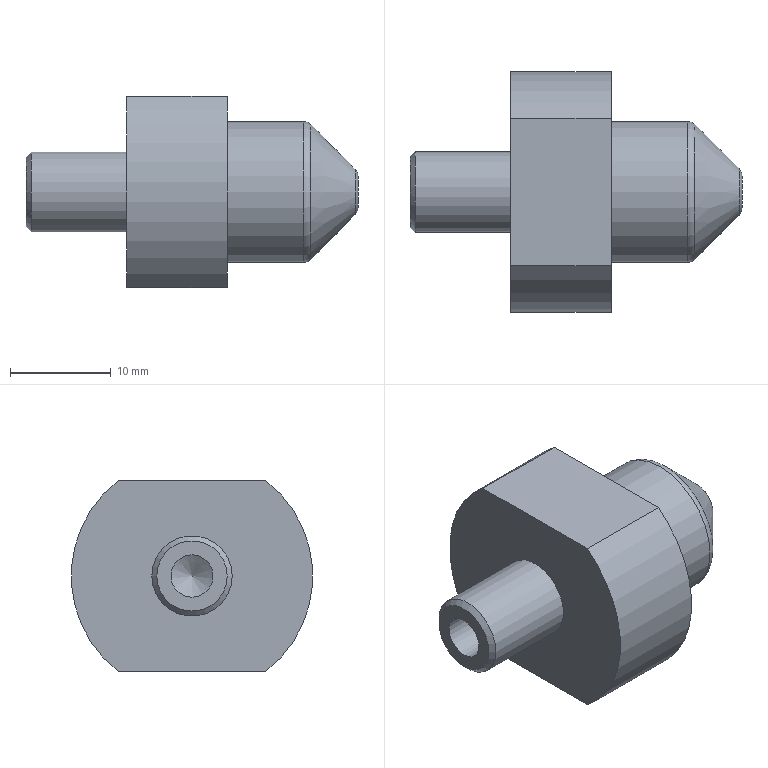Part | NX | features BREP 1 | 1 solid | 16 faces | box 33 x 24 x 19 mm | volume 5927 mm3 | plane 6 | cylinder 5 | cone 3 | torus 2 | commonest cylinder face diameters 24 x2 4.2 x1 8 x1 14 x1
STEP:
#1=CARTESIAN_POINT('',(3.5,-7.331,-9.5));
#2=VERTEX_POINT('',#1);
#3=CARTESIAN_POINT('',(3.5,-7.331,9.5));
#4=VERTEX_POINT('',#3);
#5=CARTESIAN_POINT('',(3.5,0.,0.));
#6=DIRECTION('',(-1.,0.,0.));
#7=DIRECTION('',(0.,-1.,0.));
#8=AXIS2_PLACEMENT_3D('',#5,#6,#7);
#9=CIRCLE('',#8,12.);
#10=EDGE_CURVE('',#2,#4,#9,.T.);
#11=ORIENTED_EDGE('',*,*,#10,.T.);
#12=CARTESIAN_POINT('',(-6.5,-7.331,9.5));
#13=VERTEX_POINT('',#12);
#14=CARTESIAN_POINT('',(-16.5,-7.331,9.5));
#15=DIRECTION('',(-1.,0.,0.));
#16=VECTOR('',#15,1000.);
#17=LINE('',#14,#16);
#18=EDGE_CURVE('',#4,#13,#17,.T.);
#19=ORIENTED_EDGE('',*,*,#18,.T.);
#20=CARTESIAN_POINT('',(-6.5,-7.331,-9.5));
#21=VERTEX_POINT('',#20);
#22=CARTESIAN_POINT('',(-6.5,0.,0.));
#23=DIRECTION('',(-1.,0.,0.));
#24=DIRECTION('',(0.,-1.,0.));
#25=AXIS2_PLACEMENT_3D('',#22,#23,#24);
#26=CIRCLE('',#25,12.);
#27=EDGE_CURVE('',#21,#13,#26,.T.);
#28=ORIENTED_EDGE('',*,*,#27,.F.);
#29=CARTESIAN_POINT('',(-16.5,-7.331,-9.5));
#30=DIRECTION('',(1.,0.,0.));
#31=VECTOR('',#30,1000.);
#32=LINE('',#29,#31);
#33=EDGE_CURVE('',#21,#2,#32,.T.);
#34=ORIENTED_EDGE('',*,*,#33,.T.);
#35=EDGE_LOOP('',(#11,#19,#28,#34));
#36=FACE_BOUND('',#35,.T.);
#37=CARTESIAN_POINT('',(-16.5,0.,0.));
#38=DIRECTION('',(-1.,0.,0.));
#39=DIRECTION('',(0.,1.,0.));
#40=AXIS2_PLACEMENT_3D('',#37,#38,#39);
#41=CYLINDRICAL_SURFACE('',#40,12.);
#42=ADVANCED_FACE('',(#36),#41,.T.);
#43=CARTESIAN_POINT('',(-16.5,3.5,0.));
#44=VERTEX_POINT('',#43);
#45=CARTESIAN_POINT('',(-16.5,0.,0.));
#46=DIRECTION('',(-1.,0.,0.));
#47=DIRECTION('',(0.,1.,0.));
#48=AXIS2_PLACEMENT_3D('',#45,#46,#47);
#49=CIRCLE('',#48,3.5);
#50=EDGE_CURVE('',#44,#44,#49,.T.);
#51=ORIENTED_EDGE('',*,*,#50,.T.);
#52=EDGE_LOOP('',(#51));
#53=FACE_BOUND('',#52,.T.);
#54=CARTESIAN_POINT('',(-16.5,0.,2.1));
#55=VERTEX_POINT('',#54);
#56=CARTESIAN_POINT('',(-16.5,0.,0.));
#57=DIRECTION('',(-1.,0.,0.));
#58=DIRECTION('',(0.,0.,1.));
#59=AXIS2_PLACEMENT_3D('',#56,#57,#58);
#60=CIRCLE('',#59,2.1);
#61=EDGE_CURVE('',#55,#55,#60,.T.);
#62=ORIENTED_EDGE('',*,*,#61,.F.);
#63=EDGE_LOOP('',(#62));
#64=FACE_BOUND('',#63,.T.);
#65=CARTESIAN_POINT('',(-16.5,4.,0.));
#66=DIRECTION('',(1.,0.,0.));
#67=DIRECTION('',(0.,-1.,0.));
#68=AXIS2_PLACEMENT_3D('',#65,#66,#67);
#69=PLANE('',#68);
#70=ADVANCED_FACE('',(#53,#64),#69,.F.);
#71=CARTESIAN_POINT('',(16.5,-1.586,0.));
#72=VERTEX_POINT('',#71);
#73=CARTESIAN_POINT('',(16.5,0.,0.));
#74=DIRECTION('',(1.,0.,0.));
#75=DIRECTION('',(0.,-1.,0.));
#76=AXIS2_PLACEMENT_3D('',#73,#74,#75);
#77=CIRCLE('',#76,1.586);
#78=EDGE_CURVE('',#72,#72,#77,.T.);
#79=ORIENTED_EDGE('',*,*,#78,.T.);
#80=EDGE_LOOP('',(#79));
#81=FACE_BOUND('',#80,.T.);
#82=CARTESIAN_POINT('',(16.5,0.,0.));
#83=DIRECTION('',(-1.,0.,0.));
#84=DIRECTION('',(0.,1.,0.));
#85=AXIS2_PLACEMENT_3D('',#82,#83,#84);
#86=PLANE('',#85);
#87=ADVANCED_FACE('',(#81),#86,.F.);
#88=CARTESIAN_POINT('',(16.207,2.293,0.));
#89=VERTEX_POINT('',#88);
#90=CARTESIAN_POINT('',(16.207,0.,0.));
#91=DIRECTION('',(-1.,0.,0.));
#92=DIRECTION('',(0.,1.,0.));
#93=AXIS2_PLACEMENT_3D('',#90,#91,#92);
#94=CIRCLE('',#93,2.293);
#95=EDGE_CURVE('',#89,#89,#94,.T.);
#96=ORIENTED_EDGE('',*,*,#95,.T.);
#97=EDGE_LOOP('',(#96));
#98=FACE_BOUND('',#97,.T.);
#99=CARTESIAN_POINT('',(11.793,6.707,0.));
#100=VERTEX_POINT('',#99);
#101=CARTESIAN_POINT('',(11.793,0.,0.));
#102=DIRECTION('',(1.,0.,0.));
#103=DIRECTION('',(0.,1.,0.));
#104=AXIS2_PLACEMENT_3D('',#101,#102,#103);
#105=CIRCLE('',#104,6.707);
#106=EDGE_CURVE('',#100,#100,#105,.T.);
#107=ORIENTED_EDGE('',*,*,#106,.T.);
#108=EDGE_LOOP('',(#107));
#109=FACE_BOUND('',#108,.T.);
#110=CARTESIAN_POINT('',(16.5,0.,0.));
#111=DIRECTION('',(-1.,0.,0.));
#112=DIRECTION('',(0.,1.,0.));
#113=AXIS2_PLACEMENT_3D('',#110,#111,#112);
#114=CONICAL_SURFACE('',#113,2.,0.7854);
#115=ADVANCED_FACE('',(#98,#109),#114,.T.);
#116=CARTESIAN_POINT('',(11.086,7.,0.));
#117=VERTEX_POINT('',#116);
#118=CARTESIAN_POINT('',(11.086,0.,0.));
#119=DIRECTION('',(-1.,0.,0.));
#120=DIRECTION('',(0.,1.,0.));
#121=AXIS2_PLACEMENT_3D('',#118,#119,#120);
#122=CIRCLE('',#121,7.);
#123=EDGE_CURVE('',#117,#117,#122,.T.);
#124=ORIENTED_EDGE('',*,*,#123,.T.);
#125=EDGE_LOOP('',(#124));
#126=FACE_BOUND('',#125,.T.);
#127=CARTESIAN_POINT('',(3.5,-7.,0.));
#128=VERTEX_POINT('',#127);
#129=CARTESIAN_POINT('',(3.5,0.,0.));
#130=DIRECTION('',(-1.,0.,0.));
#131=DIRECTION('',(0.,-1.,0.));
#132=AXIS2_PLACEMENT_3D('',#129,#130,#131);
#133=CIRCLE('',#132,7.);
#134=EDGE_CURVE('',#128,#128,#133,.T.);
#135=ORIENTED_EDGE('',*,*,#134,.F.);
#136=EDGE_LOOP('',(#135));
#137=FACE_BOUND('',#136,.T.);
#138=CARTESIAN_POINT('',(-16.5,0.,0.));
#139=DIRECTION('',(-1.,0.,0.));
#140=DIRECTION('',(0.,1.,0.));
#141=AXIS2_PLACEMENT_3D('',#138,#139,#140);
#142=CYLINDRICAL_SURFACE('',#141,7.);
#143=ADVANCED_FACE('',(#126,#137),#142,.T.);
#144=CARTESIAN_POINT('',(3.5,7.331,9.5));
#145=VERTEX_POINT('',#144);
#146=CARTESIAN_POINT('',(3.5,7.331,-9.5));
#147=VERTEX_POINT('',#146);
#148=CARTESIAN_POINT('',(3.5,0.,0.));
#149=DIRECTION('',(-1.,0.,0.));
#150=DIRECTION('',(0.,-1.,0.));
#151=AXIS2_PLACEMENT_3D('',#148,#149,#150);
#152=CIRCLE('',#151,12.);
#153=EDGE_CURVE('',#145,#147,#152,.T.);
#154=ORIENTED_EDGE('',*,*,#153,.F.);
#155=CARTESIAN_POINT('',(3.5,-10.985,9.5));
#156=DIRECTION('',(0.,1.,0.));
#157=VECTOR('',#156,1000.);
#158=LINE('',#155,#157);
#159=EDGE_CURVE('',#4,#145,#158,.T.);
#160=ORIENTED_EDGE('',*,*,#159,.F.);
#161=ORIENTED_EDGE('',*,*,#10,.F.);
#162=CARTESIAN_POINT('',(3.5,-9.895,-9.5));
#163=DIRECTION('',(0.,-1.,0.));
#164=VECTOR('',#163,1000.);
#165=LINE('',#162,#164);
#166=EDGE_CURVE('',#147,#2,#165,.T.);
#167=ORIENTED_EDGE('',*,*,#166,.F.);
#168=EDGE_LOOP('',(#154,#160,#161,#167));
#169=FACE_BOUND('',#168,.T.);
#170=ORIENTED_EDGE('',*,*,#134,.T.);
#171=EDGE_LOOP('',(#170));
#172=FACE_BOUND('',#171,.T.);
#173=CARTESIAN_POINT('',(3.5,7.,0.));
#174=DIRECTION('',(-1.,0.,0.));
#175=DIRECTION('',(0.,1.,0.));
#176=AXIS2_PLACEMENT_3D('',#173,#174,#175);
#177=PLANE('',#176);
#178=ADVANCED_FACE('',(#169,#172),#177,.F.);
#179=CARTESIAN_POINT('',(-6.5,7.331,9.5));
#180=VERTEX_POINT('',#179);
#181=CARTESIAN_POINT('',(-6.5,7.331,-9.5));
#182=VERTEX_POINT('',#181);
#183=CARTESIAN_POINT('',(-6.5,0.,0.));
#184=DIRECTION('',(-1.,0.,0.));
#185=DIRECTION('',(0.,-1.,0.));
#186=AXIS2_PLACEMENT_3D('',#183,#184,#185);
#187=CIRCLE('',#186,12.);
#188=EDGE_CURVE('',#180,#182,#187,.T.);
#189=ORIENTED_EDGE('',*,*,#188,.F.);
#190=CARTESIAN_POINT('',(-16.5,7.331,9.5));
#191=DIRECTION('',(1.,0.,0.));
#192=VECTOR('',#191,1000.);
#193=LINE('',#190,#192);
#194=EDGE_CURVE('',#180,#145,#193,.T.);
#195=ORIENTED_EDGE('',*,*,#194,.T.);
#196=ORIENTED_EDGE('',*,*,#153,.T.);
#197=CARTESIAN_POINT('',(-16.5,7.331,-9.5));
#198=DIRECTION('',(-1.,0.,0.));
#199=VECTOR('',#198,1000.);
#200=LINE('',#197,#199);
#201=EDGE_CURVE('',#147,#182,#200,.T.);
#202=ORIENTED_EDGE('',*,*,#201,.T.);
#203=EDGE_LOOP('',(#189,#195,#196,#202));
#204=FACE_BOUND('',#203,.T.);
#205=CARTESIAN_POINT('',(-16.5,0.,0.));
#206=DIRECTION('',(-1.,0.,0.));
#207=DIRECTION('',(0.,1.,0.));
#208=AXIS2_PLACEMENT_3D('',#205,#206,#207);
#209=CYLINDRICAL_SURFACE('',#208,12.);
#210=ADVANCED_FACE('',(#204),#209,.T.);
#211=CARTESIAN_POINT('',(-6.5,-4.,0.));
#212=VERTEX_POINT('',#211);
#213=CARTESIAN_POINT('',(-6.5,0.,0.));
#214=DIRECTION('',(-1.,0.,0.));
#215=DIRECTION('',(0.,-1.,0.));
#216=AXIS2_PLACEMENT_3D('',#213,#214,#215);
#217=CIRCLE('',#216,4.);
#218=EDGE_CURVE('',#212,#212,#217,.T.);
#219=ORIENTED_EDGE('',*,*,#218,.F.);
#220=EDGE_LOOP('',(#219));
#221=FACE_BOUND('',#220,.T.);
#222=ORIENTED_EDGE('',*,*,#27,.T.);
#223=CARTESIAN_POINT('',(-6.5,12.,9.5));
#224=DIRECTION('',(0.,1.,0.));
#225=VECTOR('',#224,1000.);
#226=LINE('',#223,#225);
#227=EDGE_CURVE('',#13,#180,#226,.T.);
#228=ORIENTED_EDGE('',*,*,#227,.T.);
#229=ORIENTED_EDGE('',*,*,#188,.T.);
#230=CARTESIAN_POINT('',(-6.5,12.,-9.5));
#231=DIRECTION('',(0.,-1.,0.));
#232=VECTOR('',#231,1000.);
#233=LINE('',#230,#232);
#234=EDGE_CURVE('',#182,#21,#233,.T.);
#235=ORIENTED_EDGE('',*,*,#234,.T.);
#236=EDGE_LOOP('',(#222,#228,#229,#235));
#237=FACE_BOUND('',#236,.T.);
#238=CARTESIAN_POINT('',(-6.5,12.,0.));
#239=DIRECTION('',(1.,0.,0.));
#240=DIRECTION('',(0.,-1.,0.));
#241=AXIS2_PLACEMENT_3D('',#238,#239,#240);
#242=PLANE('',#241);
#243=ADVANCED_FACE('',(#221,#237),#242,.F.);
#244=CARTESIAN_POINT('',(-16.,4.,0.));
#245=VERTEX_POINT('',#244);
#246=CARTESIAN_POINT('',(-16.,0.,0.));
#247=DIRECTION('',(1.,0.,0.));
#248=DIRECTION('',(0.,1.,0.));
#249=AXIS2_PLACEMENT_3D('',#246,#247,#248);
#250=CIRCLE('',#249,4.);
#251=EDGE_CURVE('',#245,#245,#250,.T.);
#252=ORIENTED_EDGE('',*,*,#251,.T.);
#253=EDGE_LOOP('',(#252));
#254=FACE_BOUND('',#253,.T.);
#255=ORIENTED_EDGE('',*,*,#218,.T.);
#256=EDGE_LOOP('',(#255));
#257=FACE_BOUND('',#256,.T.);
#258=CARTESIAN_POINT('',(-16.5,0.,0.));
#259=DIRECTION('',(-1.,0.,0.));
#260=DIRECTION('',(0.,1.,0.));
#261=AXIS2_PLACEMENT_3D('',#258,#259,#260);
#262=CYLINDRICAL_SURFACE('',#261,4.);
#263=ADVANCED_FACE('',(#254,#257),#262,.T.);
#264=ORIENTED_EDGE('',*,*,#78,.F.);
#265=EDGE_LOOP('',(#264));
#266=FACE_BOUND('',#265,.T.);
#267=ORIENTED_EDGE('',*,*,#95,.F.);
#268=EDGE_LOOP('',(#267));
#269=FACE_BOUND('',#268,.T.);
#270=CARTESIAN_POINT('',(15.5,0.,0.));
#271=DIRECTION('',(-1.,0.,0.));
#272=DIRECTION('',(0.,1.,0.));
#273=AXIS2_PLACEMENT_3D('',#270,#271,#272);
#274=TOROIDAL_SURFACE('',#273,1.586,1.);
#275=ADVANCED_FACE('',(#266,#269),#274,.T.);
#276=ORIENTED_EDGE('',*,*,#106,.F.);
#277=EDGE_LOOP('',(#276));
#278=FACE_BOUND('',#277,.T.);
#279=ORIENTED_EDGE('',*,*,#123,.F.);
#280=EDGE_LOOP('',(#279));
#281=FACE_BOUND('',#280,.T.);
#282=CARTESIAN_POINT('',(11.086,0.,0.));
#283=DIRECTION('',(1.,0.,0.));
#284=DIRECTION('',(0.,-1.,0.));
#285=AXIS2_PLACEMENT_3D('',#282,#283,#284);
#286=TOROIDAL_SURFACE('',#285,6.,1.);
#287=ADVANCED_FACE('',(#278,#281),#286,.T.);
#288=CARTESIAN_POINT('',(-2.838,0.,0.));
#289=VERTEX_POINT('',#288);
#290=VERTEX_LOOP('',#289);
#291=FACE_BOUND('',#290,.T.);
#292=CARTESIAN_POINT('',(-4.1,0.,2.1));
#293=VERTEX_POINT('',#292);
#294=CARTESIAN_POINT('',(-4.1,0.,0.));
#295=DIRECTION('',(-1.,0.,0.));
#296=DIRECTION('',(0.,0.,1.));
#297=AXIS2_PLACEMENT_3D('',#294,#295,#296);
#298=CIRCLE('',#297,2.1);
#299=EDGE_CURVE('',#293,#293,#298,.T.);
#300=ORIENTED_EDGE('',*,*,#299,.T.);
#301=EDGE_LOOP('',(#300));
#302=FACE_BOUND('',#301,.T.);
#303=CARTESIAN_POINT('',(-4.1,0.,0.));
#304=DIRECTION('',(-1.,0.,0.));
#305=DIRECTION('',(0.,0.,-1.));
#306=AXIS2_PLACEMENT_3D('',#303,#304,#305);
#307=CONICAL_SURFACE('',#306,2.1,1.03);
#308=ADVANCED_FACE('',(#291,#302),#307,.F.);
#309=ORIENTED_EDGE('',*,*,#299,.F.);
#310=EDGE_LOOP('',(#309));
#311=FACE_BOUND('',#310,.T.);
#312=ORIENTED_EDGE('',*,*,#61,.T.);
#313=EDGE_LOOP('',(#312));
#314=FACE_BOUND('',#313,.T.);
#315=CARTESIAN_POINT('',(-16.5,0.,0.));
#316=DIRECTION('',(-1.,0.,0.));
#317=DIRECTION('',(0.,0.,-1.));
#318=AXIS2_PLACEMENT_3D('',#315,#316,#317);
#319=CYLINDRICAL_SURFACE('',#318,2.1);
#320=ADVANCED_FACE('',(#311,#314),#319,.F.);
#321=ORIENTED_EDGE('',*,*,#251,.F.);
#322=EDGE_LOOP('',(#321));
#323=FACE_BOUND('',#322,.T.);
#324=ORIENTED_EDGE('',*,*,#50,.F.);
#325=EDGE_LOOP('',(#324));
#326=FACE_BOUND('',#325,.T.);
#327=CARTESIAN_POINT('',(-16.5,0.,0.));
#328=DIRECTION('',(1.,0.,0.));
#329=DIRECTION('',(0.,-1.,0.));
#330=AXIS2_PLACEMENT_3D('',#327,#328,#329);
#331=CONICAL_SURFACE('',#330,3.5,0.7854);
#332=ADVANCED_FACE('',(#323,#326),#331,.T.);
#333=ORIENTED_EDGE('',*,*,#166,.T.);
#334=ORIENTED_EDGE('',*,*,#33,.F.);
#335=ORIENTED_EDGE('',*,*,#234,.F.);
#336=ORIENTED_EDGE('',*,*,#201,.F.);
#337=EDGE_LOOP('',(#333,#334,#335,#336));
#338=FACE_BOUND('',#337,.T.);
#339=CARTESIAN_POINT('',(-6.5,-9.895,-9.5));
#340=DIRECTION('',(0.,0.,1.));
#341=DIRECTION('',(-1.,0.,0.));
#342=AXIS2_PLACEMENT_3D('',#339,#340,#341);
#343=PLANE('',#342);
#344=ADVANCED_FACE('',(#338),#343,.F.);
#345=ORIENTED_EDGE('',*,*,#159,.T.);
#346=ORIENTED_EDGE('',*,*,#194,.F.);
#347=ORIENTED_EDGE('',*,*,#227,.F.);
#348=ORIENTED_EDGE('',*,*,#18,.F.);
#349=EDGE_LOOP('',(#345,#346,#347,#348));
#350=FACE_BOUND('',#349,.T.);
#351=CARTESIAN_POINT('',(-6.5,-10.985,9.5));
#352=DIRECTION('',(0.,0.,-1.));
#353=DIRECTION('',(1.,0.,0.));
#354=AXIS2_PLACEMENT_3D('',#351,#352,#353);
#355=PLANE('',#354);
#356=ADVANCED_FACE('',(#350),#355,.F.);
#357=CLOSED_SHELL('',(#42,#70,#87,#115,#143,#178,#210,#243,#263,#275,#287,#308,#320,#332,#344,#356));
#358=MANIFOLD_SOLID_BREP('',#357);
#359=(LENGTH_UNIT()NAMED_UNIT(*)SI_UNIT(.MILLI.,.METRE.));
#360=UNCERTAINTY_MEASURE_WITH_UNIT(LENGTH_MEASURE(0.00001),#359,'','');
#361=(NAMED_UNIT(*)PLANE_ANGLE_UNIT()SI_UNIT($,.RADIAN.));
#362=(NAMED_UNIT(*)SI_UNIT($,.STERADIAN.)SOLID_ANGLE_UNIT());
#363=(GEOMETRIC_REPRESENTATION_CONTEXT(3)GLOBAL_UNCERTAINTY_ASSIGNED_CONTEXT((#360))GLOBAL_UNIT_ASSIGNED_CONTEXT((#359,#361,#362))REPRESENTATION_CONTEXT('',''));
#364=ADVANCED_BREP_SHAPE_REPRESENTATION('',(#358),#363);